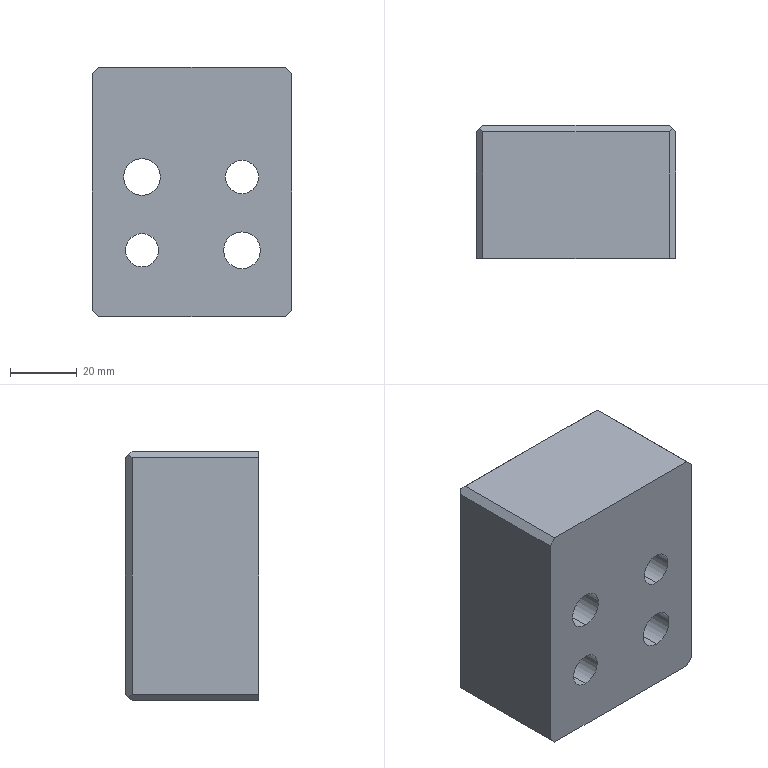Part | Creo | 1 solid | 28 faces | box 60 x 40 x 75 mm | volume 162492 mm3 | plane 16 | cylinder 12 | commonest cylinder face diameters 10 x4 11 x4 16.8 x4
STEP:
#1=CARTESIAN_POINT('',(-118.,350.,-254.5));
#2=VERTEX_POINT('',#1);
#3=CARTESIAN_POINT('',(-118.,350.,-243.5));
#4=VERTEX_POINT('',#3);
#5=CARTESIAN_POINT('',(-118.,350.,-249.));
#6=DIRECTION('',(0.,1.,0.));
#7=DIRECTION('',(0.,0.,-1.));
#8=AXIS2_PLACEMENT_3D('',#5,#6,#7);
#9=CIRCLE('',#8,5.5);
#10=EDGE_CURVE('',#2,#4,#9,.T.);
#11=ORIENTED_EDGE('',*,*,#10,.T.);
#12=CARTESIAN_POINT('',(-118.,379.,-243.5));
#13=VERTEX_POINT('',#12);
#14=CARTESIAN_POINT('',(-118.,350.,-243.5));
#15=DIRECTION('',(0.,1.,0.));
#16=VECTOR('',#15,29.);
#17=LINE('',#14,#16);
#18=EDGE_CURVE('',#4,#13,#17,.T.);
#19=ORIENTED_EDGE('',*,*,#18,.T.);
#20=CARTESIAN_POINT('',(-118.,379.,-254.5));
#21=VERTEX_POINT('',#20);
#22=CARTESIAN_POINT('',(-118.,379.,-249.));
#23=DIRECTION('',(0.,-1.,0.));
#24=DIRECTION('',(0.,0.,1.));
#25=AXIS2_PLACEMENT_3D('',#22,#23,#24);
#26=CIRCLE('',#25,5.5);
#27=EDGE_CURVE('',#13,#21,#26,.T.);
#28=ORIENTED_EDGE('',*,*,#27,.T.);
#29=CARTESIAN_POINT('',(-118.,350.,-254.5));
#30=DIRECTION('',(0.,1.,0.));
#31=VECTOR('',#30,29.);
#32=LINE('',#29,#31);
#33=EDGE_CURVE('',#2,#21,#32,.T.);
#34=ORIENTED_EDGE('',*,*,#33,.F.);
#35=EDGE_LOOP('',(#11,#19,#28,#34));
#36=FACE_OUTER_BOUND('',#35,.F.);
#37=CARTESIAN_POINT('',(-118.,390.,-249.));
#38=DIRECTION('',(0.,1.,0.));
#39=DIRECTION('',(0.,0.,-1.));
#40=AXIS2_PLACEMENT_3D('',#37,#38,#39);
#41=CYLINDRICAL_SURFACE('',#40,5.5);
#42=ADVANCED_FACE('',(#36),#41,.F.);
#43=CARTESIAN_POINT('',(-73.,350.,-289.));
#44=VERTEX_POINT('',#43);
#45=CARTESIAN_POINT('',(-73.,350.,-218.));
#46=VERTEX_POINT('',#45);
#47=CARTESIAN_POINT('',(-73.,350.,-289.));
#48=DIRECTION('',(0.,0.,1.));
#49=VECTOR('',#48,71.);
#50=LINE('',#47,#49);
#51=EDGE_CURVE('',#44,#46,#50,.T.);
#52=ORIENTED_EDGE('',*,*,#51,.F.);
#53=CARTESIAN_POINT('',(-75.,350.,-291.));
#54=VERTEX_POINT('',#53);
#55=CARTESIAN_POINT('',(-75.,350.,-291.));
#56=DIRECTION('',(0.7071,0.,0.7071));
#57=VECTOR('',#56,2.828);
#58=LINE('',#55,#57);
#59=EDGE_CURVE('',#54,#44,#58,.T.);
#60=ORIENTED_EDGE('',*,*,#59,.F.);
#61=CARTESIAN_POINT('',(-131.,350.,-291.));
#62=VERTEX_POINT('',#61);
#63=CARTESIAN_POINT('',(-131.,350.,-291.));
#64=DIRECTION('',(1.,0.,0.));
#65=VECTOR('',#64,56.);
#66=LINE('',#63,#65);
#67=EDGE_CURVE('',#62,#54,#66,.T.);
#68=ORIENTED_EDGE('',*,*,#67,.F.);
#69=CARTESIAN_POINT('',(-133.,350.,-289.));
#70=VERTEX_POINT('',#69);
#71=CARTESIAN_POINT('',(-133.,350.,-289.));
#72=DIRECTION('',(0.7071,0.,-0.7071));
#73=VECTOR('',#72,2.828);
#74=LINE('',#71,#73);
#75=EDGE_CURVE('',#70,#62,#74,.T.);
#76=ORIENTED_EDGE('',*,*,#75,.F.);
#77=CARTESIAN_POINT('',(-133.,350.,-218.));
#78=VERTEX_POINT('',#77);
#79=CARTESIAN_POINT('',(-133.,350.,-218.));
#80=DIRECTION('',(0.,0.,-1.));
#81=VECTOR('',#80,71.);
#82=LINE('',#79,#81);
#83=EDGE_CURVE('',#78,#70,#82,.T.);
#84=ORIENTED_EDGE('',*,*,#83,.F.);
#85=CARTESIAN_POINT('',(-131.,350.,-216.));
#86=VERTEX_POINT('',#85);
#87=CARTESIAN_POINT('',(-131.,350.,-216.));
#88=DIRECTION('',(-0.7071,0.,-0.7071));
#89=VECTOR('',#88,2.828);
#90=LINE('',#87,#89);
#91=EDGE_CURVE('',#86,#78,#90,.T.);
#92=ORIENTED_EDGE('',*,*,#91,.F.);
#93=CARTESIAN_POINT('',(-75.,350.,-216.));
#94=VERTEX_POINT('',#93);
#95=CARTESIAN_POINT('',(-75.,350.,-216.));
#96=DIRECTION('',(-1.,0.,0.));
#97=VECTOR('',#96,56.);
#98=LINE('',#95,#97);
#99=EDGE_CURVE('',#94,#86,#98,.T.);
#100=ORIENTED_EDGE('',*,*,#99,.F.);
#101=CARTESIAN_POINT('',(-73.,350.,-218.));
#102=DIRECTION('',(-0.7071,0.,0.7071));
#103=VECTOR('',#102,2.828);
#104=LINE('',#101,#103);
#105=EDGE_CURVE('',#46,#94,#104,.T.);
#106=ORIENTED_EDGE('',*,*,#105,.F.);
#107=EDGE_LOOP('',(#52,#60,#68,#76,#84,#92,#100,#106));
#108=FACE_OUTER_BOUND('',#107,.F.);
#109=ORIENTED_EDGE('',*,*,#10,.F.);
#110=CARTESIAN_POINT('',(-118.,350.,-249.));
#111=DIRECTION('',(0.,1.,0.));
#112=DIRECTION('',(0.,0.,1.));
#113=AXIS2_PLACEMENT_3D('',#110,#111,#112);
#114=CIRCLE('',#113,5.5);
#115=EDGE_CURVE('',#4,#2,#114,.T.);
#116=ORIENTED_EDGE('',*,*,#115,.F.);
#117=EDGE_LOOP('',(#109,#116));
#118=FACE_BOUND('',#117,.F.);
#119=CARTESIAN_POINT('',(-88.,350.,-276.5));
#120=VERTEX_POINT('',#119);
#121=CARTESIAN_POINT('',(-88.,350.,-265.5));
#122=VERTEX_POINT('',#121);
#123=CARTESIAN_POINT('',(-88.,350.,-271.));
#124=DIRECTION('',(0.,1.,0.));
#125=DIRECTION('',(0.,0.,-1.));
#126=AXIS2_PLACEMENT_3D('',#123,#124,#125);
#127=CIRCLE('',#126,5.5);
#128=EDGE_CURVE('',#120,#122,#127,.T.);
#129=ORIENTED_EDGE('',*,*,#128,.F.);
#130=CARTESIAN_POINT('',(-88.,350.,-271.));
#131=DIRECTION('',(0.,1.,0.));
#132=DIRECTION('',(0.,0.,1.));
#133=AXIS2_PLACEMENT_3D('',#130,#131,#132);
#134=CIRCLE('',#133,5.5);
#135=EDGE_CURVE('',#122,#120,#134,.T.);
#136=ORIENTED_EDGE('',*,*,#135,.F.);
#137=EDGE_LOOP('',(#129,#136));
#138=FACE_BOUND('',#137,.F.);
#139=CARTESIAN_POINT('',(-118.,350.,-276.));
#140=VERTEX_POINT('',#139);
#141=CARTESIAN_POINT('',(-118.,350.,-266.));
#142=VERTEX_POINT('',#141);
#143=CARTESIAN_POINT('',(-118.,350.,-271.));
#144=DIRECTION('',(0.,1.,0.));
#145=DIRECTION('',(0.,0.,-1.));
#146=AXIS2_PLACEMENT_3D('',#143,#144,#145);
#147=CIRCLE('',#146,5.);
#148=EDGE_CURVE('',#140,#142,#147,.T.);
#149=ORIENTED_EDGE('',*,*,#148,.F.);
#150=CARTESIAN_POINT('',(-118.,350.,-271.));
#151=DIRECTION('',(0.,1.,0.));
#152=DIRECTION('',(0.,0.,1.));
#153=AXIS2_PLACEMENT_3D('',#150,#151,#152);
#154=CIRCLE('',#153,5.);
#155=EDGE_CURVE('',#142,#140,#154,.T.);
#156=ORIENTED_EDGE('',*,*,#155,.F.);
#157=EDGE_LOOP('',(#149,#156));
#158=FACE_BOUND('',#157,.F.);
#159=CARTESIAN_POINT('',(-88.,350.,-254.));
#160=VERTEX_POINT('',#159);
#161=CARTESIAN_POINT('',(-88.,350.,-244.));
#162=VERTEX_POINT('',#161);
#163=CARTESIAN_POINT('',(-88.,350.,-249.));
#164=DIRECTION('',(0.,1.,0.));
#165=DIRECTION('',(0.,0.,-1.));
#166=AXIS2_PLACEMENT_3D('',#163,#164,#165);
#167=CIRCLE('',#166,5.);
#168=EDGE_CURVE('',#160,#162,#167,.T.);
#169=ORIENTED_EDGE('',*,*,#168,.F.);
#170=CARTESIAN_POINT('',(-88.,350.,-249.));
#171=DIRECTION('',(0.,1.,0.));
#172=DIRECTION('',(0.,0.,1.));
#173=AXIS2_PLACEMENT_3D('',#170,#171,#172);
#174=CIRCLE('',#173,5.);
#175=EDGE_CURVE('',#162,#160,#174,.T.);
#176=ORIENTED_EDGE('',*,*,#175,.F.);
#177=EDGE_LOOP('',(#169,#176));
#178=FACE_BOUND('',#177,.F.);
#179=CARTESIAN_POINT('',(321.5,350.,45.));
#180=DIRECTION('',(0.,1.,0.));
#181=DIRECTION('',(0.,0.,-1.));
#182=AXIS2_PLACEMENT_3D('',#179,#180,#181);
#183=PLANE('',#182);
#184=ADVANCED_FACE('',(#108,#118,#138,#158,#178),#183,.F.);
#185=CARTESIAN_POINT('',(-73.,388.,-289.));
#186=VERTEX_POINT('',#185);
#187=CARTESIAN_POINT('',(-73.,388.,-218.));
#188=VERTEX_POINT('',#187);
#189=CARTESIAN_POINT('',(-73.,388.,-289.));
#190=DIRECTION('',(0.,0.,1.));
#191=VECTOR('',#190,71.);
#192=LINE('',#189,#191);
#193=EDGE_CURVE('',#186,#188,#192,.T.);
#194=ORIENTED_EDGE('',*,*,#193,.F.);
#195=CARTESIAN_POINT('',(-73.,350.,-289.));
#196=DIRECTION('',(0.,1.,0.));
#197=VECTOR('',#196,38.);
#198=LINE('',#195,#197);
#199=EDGE_CURVE('',#44,#186,#198,.T.);
#200=ORIENTED_EDGE('',*,*,#199,.F.);
#201=ORIENTED_EDGE('',*,*,#51,.T.);
#202=CARTESIAN_POINT('',(-73.,350.,-218.));
#203=DIRECTION('',(0.,1.,0.));
#204=VECTOR('',#203,38.);
#205=LINE('',#202,#204);
#206=EDGE_CURVE('',#46,#188,#205,.T.);
#207=ORIENTED_EDGE('',*,*,#206,.T.);
#208=EDGE_LOOP('',(#194,#200,#201,#207));
#209=FACE_OUTER_BOUND('',#208,.F.);
#210=CARTESIAN_POINT('',(-73.,350.,-216.));
#211=DIRECTION('',(1.,0.,0.));
#212=DIRECTION('',(0.,0.,1.));
#213=AXIS2_PLACEMENT_3D('',#210,#211,#212);
#214=PLANE('',#213);
#215=ADVANCED_FACE('',(#209),#214,.T.);
#216=CARTESIAN_POINT('',(-74.,389.,-217.));
#217=VERTEX_POINT('',#216);
#218=CARTESIAN_POINT('',(-75.,390.,-218.));
#219=VERTEX_POINT('',#218);
#220=CARTESIAN_POINT('',(-74.,389.,-217.));
#221=DIRECTION('',(-0.5774,0.5774,-0.5774));
#222=VECTOR('',#221,1.732);
#223=LINE('',#220,#222);
#224=EDGE_CURVE('',#217,#219,#223,.T.);
#225=ORIENTED_EDGE('',*,*,#224,.T.);
#226=CARTESIAN_POINT('',(-75.,390.,-289.));
#227=VERTEX_POINT('',#226);
#228=CARTESIAN_POINT('',(-75.,390.,-289.));
#229=DIRECTION('',(0.,0.,1.));
#230=VECTOR('',#229,71.);
#231=LINE('',#228,#230);
#232=EDGE_CURVE('',#227,#219,#231,.T.);
#233=ORIENTED_EDGE('',*,*,#232,.F.);
#234=CARTESIAN_POINT('',(-74.,389.,-290.));
#235=VERTEX_POINT('',#234);
#236=CARTESIAN_POINT('',(-75.,390.,-289.));
#237=DIRECTION('',(0.5774,-0.5774,-0.5774));
#238=VECTOR('',#237,1.732);
#239=LINE('',#236,#238);
#240=EDGE_CURVE('',#227,#235,#239,.T.);
#241=ORIENTED_EDGE('',*,*,#240,.T.);
#242=CARTESIAN_POINT('',(-74.,389.,-290.));
#243=DIRECTION('',(0.5774,-0.5774,0.5774));
#244=VECTOR('',#243,1.732);
#245=LINE('',#242,#244);
#246=EDGE_CURVE('',#235,#186,#245,.T.);
#247=ORIENTED_EDGE('',*,*,#246,.T.);
#248=ORIENTED_EDGE('',*,*,#193,.T.);
#249=CARTESIAN_POINT('',(-74.,389.,-217.));
#250=DIRECTION('',(0.5774,-0.5774,-0.5774));
#251=VECTOR('',#250,1.732);
#252=LINE('',#249,#251);
#253=EDGE_CURVE('',#217,#188,#252,.T.);
#254=ORIENTED_EDGE('',*,*,#253,.F.);
#255=EDGE_LOOP('',(#225,#233,#241,#247,#248,#254));
#256=FACE_OUTER_BOUND('',#255,.F.);
#257=CARTESIAN_POINT('',(-74.,389.,-253.5));
#258=DIRECTION('',(0.7071,0.7071,0.));
#259=DIRECTION('',(-0.7071,0.7071,0.));
#260=AXIS2_PLACEMENT_3D('',#257,#258,#259);
#261=PLANE('',#260);
#262=ADVANCED_FACE('',(#256),#261,.T.);
#263=CARTESIAN_POINT('',(-75.,388.,-216.));
#264=VERTEX_POINT('',#263);
#265=CARTESIAN_POINT('',(-75.,388.,-216.));
#266=DIRECTION('',(0.5774,0.5774,-0.5774));
#267=VECTOR('',#266,1.732);
#268=LINE('',#265,#267);
#269=EDGE_CURVE('',#264,#217,#268,.T.);
#270=ORIENTED_EDGE('',*,*,#269,.F.);
#271=CARTESIAN_POINT('',(-131.,388.,-216.));
#272=VERTEX_POINT('',#271);
#273=CARTESIAN_POINT('',(-75.,388.,-216.));
#274=DIRECTION('',(-1.,0.,0.));
#275=VECTOR('',#274,56.);
#276=LINE('',#273,#275);
#277=EDGE_CURVE('',#264,#272,#276,.T.);
#278=ORIENTED_EDGE('',*,*,#277,.T.);
#279=CARTESIAN_POINT('',(-132.,389.,-217.));
#280=VERTEX_POINT('',#279);
#281=CARTESIAN_POINT('',(-132.,389.,-217.));
#282=DIRECTION('',(0.5774,-0.5774,0.5774));
#283=VECTOR('',#282,1.732);
#284=LINE('',#281,#283);
#285=EDGE_CURVE('',#280,#272,#284,.T.);
#286=ORIENTED_EDGE('',*,*,#285,.F.);
#287=CARTESIAN_POINT('',(-131.,390.,-218.));
#288=VERTEX_POINT('',#287);
#289=CARTESIAN_POINT('',(-132.,389.,-217.));
#290=DIRECTION('',(0.5774,0.5774,-0.5774));
#291=VECTOR('',#290,1.732);
#292=LINE('',#289,#291);
#293=EDGE_CURVE('',#280,#288,#292,.T.);
#294=ORIENTED_EDGE('',*,*,#293,.T.);
#295=CARTESIAN_POINT('',(-75.,390.,-218.));
#296=DIRECTION('',(-1.,0.,0.));
#297=VECTOR('',#296,56.);
#298=LINE('',#295,#297);
#299=EDGE_CURVE('',#219,#288,#298,.T.);
#300=ORIENTED_EDGE('',*,*,#299,.F.);
#301=ORIENTED_EDGE('',*,*,#224,.F.);
#302=EDGE_LOOP('',(#270,#278,#286,#294,#300,#301));
#303=FACE_OUTER_BOUND('',#302,.F.);
#304=CARTESIAN_POINT('',(-103.,389.,-217.));
#305=DIRECTION('',(0.,0.7071,0.7071));
#306=DIRECTION('',(0.,0.7071,-0.7071));
#307=AXIS2_PLACEMENT_3D('',#304,#305,#306);
#308=PLANE('',#307);
#309=ADVANCED_FACE('',(#303),#308,.T.);
#310=ORIENTED_EDGE('',*,*,#206,.F.);
#311=ORIENTED_EDGE('',*,*,#105,.T.);
#312=CARTESIAN_POINT('',(-75.,350.,-216.));
#313=DIRECTION('',(0.,1.,0.));
#314=VECTOR('',#313,38.);
#315=LINE('',#312,#314);
#316=EDGE_CURVE('',#94,#264,#315,.T.);
#317=ORIENTED_EDGE('',*,*,#316,.T.);
#318=ORIENTED_EDGE('',*,*,#269,.T.);
#319=ORIENTED_EDGE('',*,*,#253,.T.);
#320=EDGE_LOOP('',(#310,#311,#317,#318,#319));
#321=FACE_OUTER_BOUND('',#320,.F.);
#322=CARTESIAN_POINT('',(-74.,370.,-217.));
#323=DIRECTION('',(0.7071,0.,0.7071));
#324=DIRECTION('',(-0.7071,0.,0.7071));
#325=AXIS2_PLACEMENT_3D('',#322,#323,#324);
#326=PLANE('',#325);
#327=ADVANCED_FACE('',(#321),#326,.T.);
#328=ORIENTED_EDGE('',*,*,#99,.T.);
#329=CARTESIAN_POINT('',(-131.,350.,-216.));
#330=DIRECTION('',(0.,1.,0.));
#331=VECTOR('',#330,38.);
#332=LINE('',#329,#331);
#333=EDGE_CURVE('',#86,#272,#332,.T.);
#334=ORIENTED_EDGE('',*,*,#333,.T.);
#335=ORIENTED_EDGE('',*,*,#277,.F.);
#336=ORIENTED_EDGE('',*,*,#316,.F.);
#337=EDGE_LOOP('',(#328,#334,#335,#336));
#338=FACE_OUTER_BOUND('',#337,.F.);
#339=CARTESIAN_POINT('',(-133.,350.,-216.));
#340=DIRECTION('',(0.,0.,1.));
#341=DIRECTION('',(-1.,0.,0.));
#342=AXIS2_PLACEMENT_3D('',#339,#340,#341);
#343=PLANE('',#342);
#344=ADVANCED_FACE('',(#338),#343,.T.);
#345=ORIENTED_EDGE('',*,*,#333,.F.);
#346=ORIENTED_EDGE('',*,*,#91,.T.);
#347=CARTESIAN_POINT('',(-133.,388.,-218.));
#348=VERTEX_POINT('',#347);
#349=CARTESIAN_POINT('',(-133.,350.,-218.));
#350=DIRECTION('',(0.,1.,0.));
#351=VECTOR('',#350,38.);
#352=LINE('',#349,#351);
#353=EDGE_CURVE('',#78,#348,#352,.T.);
#354=ORIENTED_EDGE('',*,*,#353,.T.);
#355=CARTESIAN_POINT('',(-133.,388.,-218.));
#356=DIRECTION('',(0.5774,0.5774,0.5774));
#357=VECTOR('',#356,1.732);
#358=LINE('',#355,#357);
#359=EDGE_CURVE('',#348,#280,#358,.T.);
#360=ORIENTED_EDGE('',*,*,#359,.T.);
#361=ORIENTED_EDGE('',*,*,#285,.T.);
#362=EDGE_LOOP('',(#345,#346,#354,#360,#361));
#363=FACE_OUTER_BOUND('',#362,.F.);
#364=CARTESIAN_POINT('',(-132.,370.,-217.));
#365=DIRECTION('',(-0.7071,0.,0.7071));
#366=DIRECTION('',(-0.7071,0.,-0.7071));
#367=AXIS2_PLACEMENT_3D('',#364,#365,#366);
#368=PLANE('',#367);
#369=ADVANCED_FACE('',(#363),#368,.T.);
#370=ORIENTED_EDGE('',*,*,#83,.T.);
#371=CARTESIAN_POINT('',(-133.,388.,-289.));
#372=VERTEX_POINT('',#371);
#373=CARTESIAN_POINT('',(-133.,350.,-289.));
#374=DIRECTION('',(0.,1.,0.));
#375=VECTOR('',#374,38.);
#376=LINE('',#373,#375);
#377=EDGE_CURVE('',#70,#372,#376,.T.);
#378=ORIENTED_EDGE('',*,*,#377,.T.);
#379=CARTESIAN_POINT('',(-133.,388.,-218.));
#380=DIRECTION('',(0.,0.,-1.));
#381=VECTOR('',#380,71.);
#382=LINE('',#379,#381);
#383=EDGE_CURVE('',#348,#372,#382,.T.);
#384=ORIENTED_EDGE('',*,*,#383,.F.);
#385=ORIENTED_EDGE('',*,*,#353,.F.);
#386=EDGE_LOOP('',(#370,#378,#384,#385));
#387=FACE_OUTER_BOUND('',#386,.F.);
#388=CARTESIAN_POINT('',(-133.,350.,-291.));
#389=DIRECTION('',(-1.,0.,0.));
#390=DIRECTION('',(0.,0.,-1.));
#391=AXIS2_PLACEMENT_3D('',#388,#389,#390);
#392=PLANE('',#391);
#393=ADVANCED_FACE('',(#387),#392,.T.);
#394=ORIENTED_EDGE('',*,*,#377,.F.);
#395=ORIENTED_EDGE('',*,*,#75,.T.);
#396=CARTESIAN_POINT('',(-131.,388.,-291.));
#397=VERTEX_POINT('',#396);
#398=CARTESIAN_POINT('',(-131.,350.,-291.));
#399=DIRECTION('',(0.,1.,0.));
#400=VECTOR('',#399,38.);
#401=LINE('',#398,#400);
#402=EDGE_CURVE('',#62,#397,#401,.T.);
#403=ORIENTED_EDGE('',*,*,#402,.T.);
#404=CARTESIAN_POINT('',(-132.,389.,-290.));
#405=VERTEX_POINT('',#404);
#406=CARTESIAN_POINT('',(-131.,388.,-291.));
#407=DIRECTION('',(-0.5774,0.5774,0.5774));
#408=VECTOR('',#407,1.732);
#409=LINE('',#406,#408);
#410=EDGE_CURVE('',#397,#405,#409,.T.);
#411=ORIENTED_EDGE('',*,*,#410,.T.);
#412=CARTESIAN_POINT('',(-132.,389.,-290.));
#413=DIRECTION('',(-0.5774,-0.5774,0.5774));
#414=VECTOR('',#413,1.732);
#415=LINE('',#412,#414);
#416=EDGE_CURVE('',#405,#372,#415,.T.);
#417=ORIENTED_EDGE('',*,*,#416,.T.);
#418=EDGE_LOOP('',(#394,#395,#403,#411,#417));
#419=FACE_OUTER_BOUND('',#418,.F.);
#420=CARTESIAN_POINT('',(-132.,370.,-290.));
#421=DIRECTION('',(-0.7071,0.,-0.7071));
#422=DIRECTION('',(0.7071,0.,-0.7071));
#423=AXIS2_PLACEMENT_3D('',#420,#421,#422);
#424=PLANE('',#423);
#425=ADVANCED_FACE('',(#419),#424,.T.);
#426=ORIENTED_EDGE('',*,*,#67,.T.);
#427=CARTESIAN_POINT('',(-75.,388.,-291.));
#428=VERTEX_POINT('',#427);
#429=CARTESIAN_POINT('',(-75.,350.,-291.));
#430=DIRECTION('',(0.,1.,0.));
#431=VECTOR('',#430,38.);
#432=LINE('',#429,#431);
#433=EDGE_CURVE('',#54,#428,#432,.T.);
#434=ORIENTED_EDGE('',*,*,#433,.T.);
#435=CARTESIAN_POINT('',(-131.,388.,-291.));
#436=DIRECTION('',(1.,0.,0.));
#437=VECTOR('',#436,56.);
#438=LINE('',#435,#437);
#439=EDGE_CURVE('',#397,#428,#438,.T.);
#440=ORIENTED_EDGE('',*,*,#439,.F.);
#441=ORIENTED_EDGE('',*,*,#402,.F.);
#442=EDGE_LOOP('',(#426,#434,#440,#441));
#443=FACE_OUTER_BOUND('',#442,.F.);
#444=CARTESIAN_POINT('',(-73.,350.,-291.));
#445=DIRECTION('',(0.,0.,-1.));
#446=DIRECTION('',(1.,0.,0.));
#447=AXIS2_PLACEMENT_3D('',#444,#445,#446);
#448=PLANE('',#447);
#449=ADVANCED_FACE('',(#443),#448,.T.);
#450=ORIENTED_EDGE('',*,*,#433,.F.);
#451=ORIENTED_EDGE('',*,*,#59,.T.);
#452=ORIENTED_EDGE('',*,*,#199,.T.);
#453=ORIENTED_EDGE('',*,*,#246,.F.);
#454=CARTESIAN_POINT('',(-74.,389.,-290.));
#455=DIRECTION('',(-0.5774,-0.5774,-0.5774));
#456=VECTOR('',#455,1.732);
#457=LINE('',#454,#456);
#458=EDGE_CURVE('',#235,#428,#457,.T.);
#459=ORIENTED_EDGE('',*,*,#458,.T.);
#460=EDGE_LOOP('',(#450,#451,#452,#453,#459));
#461=FACE_OUTER_BOUND('',#460,.F.);
#462=CARTESIAN_POINT('',(-74.,370.,-290.));
#463=DIRECTION('',(0.7071,0.,-0.7071));
#464=DIRECTION('',(0.7071,0.,0.7071));
#465=AXIS2_PLACEMENT_3D('',#462,#463,#464);
#466=PLANE('',#465);
#467=ADVANCED_FACE('',(#461),#466,.T.);
#468=ORIENTED_EDGE('',*,*,#410,.F.);
#469=ORIENTED_EDGE('',*,*,#439,.T.);
#470=ORIENTED_EDGE('',*,*,#458,.F.);
#471=ORIENTED_EDGE('',*,*,#240,.F.);
#472=CARTESIAN_POINT('',(-131.,390.,-289.));
#473=VERTEX_POINT('',#472);
#474=CARTESIAN_POINT('',(-131.,390.,-289.));
#475=DIRECTION('',(1.,0.,0.));
#476=VECTOR('',#475,56.);
#477=LINE('',#474,#476);
#478=EDGE_CURVE('',#473,#227,#477,.T.);
#479=ORIENTED_EDGE('',*,*,#478,.F.);
#480=CARTESIAN_POINT('',(-132.,389.,-290.));
#481=DIRECTION('',(0.5774,0.5774,0.5774));
#482=VECTOR('',#481,1.732);
#483=LINE('',#480,#482);
#484=EDGE_CURVE('',#405,#473,#483,.T.);
#485=ORIENTED_EDGE('',*,*,#484,.F.);
#486=EDGE_LOOP('',(#468,#469,#470,#471,#479,#485));
#487=FACE_OUTER_BOUND('',#486,.F.);
#488=CARTESIAN_POINT('',(-103.,389.,-290.));
#489=DIRECTION('',(0.,0.7071,-0.7071));
#490=DIRECTION('',(0.,-0.7071,-0.7071));
#491=AXIS2_PLACEMENT_3D('',#488,#489,#490);
#492=PLANE('',#491);
#493=ADVANCED_FACE('',(#487),#492,.T.);
#494=ORIENTED_EDGE('',*,*,#299,.T.);
#495=CARTESIAN_POINT('',(-131.,390.,-218.));
#496=DIRECTION('',(0.,0.,-1.));
#497=VECTOR('',#496,71.);
#498=LINE('',#495,#497);
#499=EDGE_CURVE('',#288,#473,#498,.T.);
#500=ORIENTED_EDGE('',*,*,#499,.T.);
#501=ORIENTED_EDGE('',*,*,#478,.T.);
#502=ORIENTED_EDGE('',*,*,#232,.T.);
#503=EDGE_LOOP('',(#494,#500,#501,#502));
#504=FACE_OUTER_BOUND('',#503,.F.);
#505=CARTESIAN_POINT('',(-126.4,390.,-249.));
#506=VERTEX_POINT('',#505);
#507=CARTESIAN_POINT('',(-118.,390.,-257.4));
#508=VERTEX_POINT('',#507);
#509=CARTESIAN_POINT('',(-118.,390.,-249.));
#510=DIRECTION('',(0.,-1.,0.));
#511=DIRECTION('',(-1.,0.,0.));
#512=AXIS2_PLACEMENT_3D('',#509,#510,#511);
#513=CIRCLE('',#512,8.4);
#514=EDGE_CURVE('',#506,#508,#513,.T.);
#515=ORIENTED_EDGE('',*,*,#514,.F.);
#516=CARTESIAN_POINT('',(-118.,390.,-240.6));
#517=VERTEX_POINT('',#516);
#518=CARTESIAN_POINT('',(-118.,390.,-249.));
#519=DIRECTION('',(0.,-1.,0.));
#520=DIRECTION('',(0.,0.,1.));
#521=AXIS2_PLACEMENT_3D('',#518,#519,#520);
#522=CIRCLE('',#521,8.4);
#523=EDGE_CURVE('',#517,#506,#522,.T.);
#524=ORIENTED_EDGE('',*,*,#523,.F.);
#525=CARTESIAN_POINT('',(-118.,390.,-249.));
#526=DIRECTION('',(0.,-1.,0.));
#527=DIRECTION('',(0.,0.,-1.));
#528=AXIS2_PLACEMENT_3D('',#525,#526,#527);
#529=CIRCLE('',#528,8.4);
#530=EDGE_CURVE('',#508,#517,#529,.T.);
#531=ORIENTED_EDGE('',*,*,#530,.F.);
#532=EDGE_LOOP('',(#515,#524,#531));
#533=FACE_BOUND('',#532,.F.);
#534=CARTESIAN_POINT('',(-96.4,390.,-271.));
#535=VERTEX_POINT('',#534);
#536=CARTESIAN_POINT('',(-88.,390.,-279.4));
#537=VERTEX_POINT('',#536);
#538=CARTESIAN_POINT('',(-88.,390.,-271.));
#539=DIRECTION('',(0.,-1.,0.));
#540=DIRECTION('',(-1.,0.,0.));
#541=AXIS2_PLACEMENT_3D('',#538,#539,#540);
#542=CIRCLE('',#541,8.4);
#543=EDGE_CURVE('',#535,#537,#542,.T.);
#544=ORIENTED_EDGE('',*,*,#543,.F.);
#545=CARTESIAN_POINT('',(-88.,390.,-262.6));
#546=VERTEX_POINT('',#545);
#547=CARTESIAN_POINT('',(-88.,390.,-271.));
#548=DIRECTION('',(0.,-1.,0.));
#549=DIRECTION('',(0.,0.,1.));
#550=AXIS2_PLACEMENT_3D('',#547,#548,#549);
#551=CIRCLE('',#550,8.4);
#552=EDGE_CURVE('',#546,#535,#551,.T.);
#553=ORIENTED_EDGE('',*,*,#552,.F.);
#554=CARTESIAN_POINT('',(-88.,390.,-271.));
#555=DIRECTION('',(0.,-1.,0.));
#556=DIRECTION('',(0.,0.,-1.));
#557=AXIS2_PLACEMENT_3D('',#554,#555,#556);
#558=CIRCLE('',#557,8.4);
#559=EDGE_CURVE('',#537,#546,#558,.T.);
#560=ORIENTED_EDGE('',*,*,#559,.F.);
#561=EDGE_LOOP('',(#544,#553,#560));
#562=FACE_BOUND('',#561,.F.);
#563=CARTESIAN_POINT('',(-118.,390.,-276.));
#564=VERTEX_POINT('',#563);
#565=CARTESIAN_POINT('',(-118.,390.,-266.));
#566=VERTEX_POINT('',#565);
#567=CARTESIAN_POINT('',(-118.,390.,-271.));
#568=DIRECTION('',(0.,-1.,0.));
#569=DIRECTION('',(0.,0.,-1.));
#570=AXIS2_PLACEMENT_3D('',#567,#568,#569);
#571=CIRCLE('',#570,5.);
#572=EDGE_CURVE('',#564,#566,#571,.T.);
#573=ORIENTED_EDGE('',*,*,#572,.F.);
#574=CARTESIAN_POINT('',(-118.,390.,-271.));
#575=DIRECTION('',(0.,-1.,0.));
#576=DIRECTION('',(0.,0.,1.));
#577=AXIS2_PLACEMENT_3D('',#574,#575,#576);
#578=CIRCLE('',#577,5.);
#579=EDGE_CURVE('',#566,#564,#578,.T.);
#580=ORIENTED_EDGE('',*,*,#579,.F.);
#581=EDGE_LOOP('',(#573,#580));
#582=FACE_BOUND('',#581,.F.);
#583=CARTESIAN_POINT('',(-88.,390.,-254.));
#584=VERTEX_POINT('',#583);
#585=CARTESIAN_POINT('',(-88.,390.,-244.));
#586=VERTEX_POINT('',#585);
#587=CARTESIAN_POINT('',(-88.,390.,-249.));
#588=DIRECTION('',(0.,-1.,0.));
#589=DIRECTION('',(0.,0.,-1.));
#590=AXIS2_PLACEMENT_3D('',#587,#588,#589);
#591=CIRCLE('',#590,5.);
#592=EDGE_CURVE('',#584,#586,#591,.T.);
#593=ORIENTED_EDGE('',*,*,#592,.F.);
#594=CARTESIAN_POINT('',(-88.,390.,-249.));
#595=DIRECTION('',(0.,-1.,0.));
#596=DIRECTION('',(0.,0.,1.));
#597=AXIS2_PLACEMENT_3D('',#594,#595,#596);
#598=CIRCLE('',#597,5.);
#599=EDGE_CURVE('',#586,#584,#598,.T.);
#600=ORIENTED_EDGE('',*,*,#599,.F.);
#601=EDGE_LOOP('',(#593,#600));
#602=FACE_BOUND('',#601,.F.);
#603=CARTESIAN_POINT('',(321.5,390.,45.));
#604=DIRECTION('',(0.,1.,0.));
#605=DIRECTION('',(0.,0.,-1.));
#606=AXIS2_PLACEMENT_3D('',#603,#604,#605);
#607=PLANE('',#606);
#608=ADVANCED_FACE('',(#504,#533,#562,#582,#602),#607,.T.);
#609=ORIENTED_EDGE('',*,*,#552,.T.);
#610=ORIENTED_EDGE('',*,*,#543,.T.);
#611=CARTESIAN_POINT('',(-88.,379.,-279.4));
#612=VERTEX_POINT('',#611);
#613=CARTESIAN_POINT('',(-88.,379.,-279.4));
#614=DIRECTION('',(0.,1.,0.));
#615=VECTOR('',#614,11.);
#616=LINE('',#613,#615);
#617=EDGE_CURVE('',#612,#537,#616,.T.);
#618=ORIENTED_EDGE('',*,*,#617,.F.);
#619=CARTESIAN_POINT('',(-96.4,379.,-271.));
#620=VERTEX_POINT('',#619);
#621=CARTESIAN_POINT('',(-88.,379.,-271.));
#622=DIRECTION('',(0.,1.,0.));
#623=DIRECTION('',(0.,0.,-1.));
#624=AXIS2_PLACEMENT_3D('',#621,#622,#623);
#625=CIRCLE('',#624,8.4);
#626=EDGE_CURVE('',#612,#620,#625,.T.);
#627=ORIENTED_EDGE('',*,*,#626,.T.);
#628=CARTESIAN_POINT('',(-88.,379.,-262.6));
#629=VERTEX_POINT('',#628);
#630=CARTESIAN_POINT('',(-88.,379.,-271.));
#631=DIRECTION('',(0.,1.,0.));
#632=DIRECTION('',(-1.,0.,0.));
#633=AXIS2_PLACEMENT_3D('',#630,#631,#632);
#634=CIRCLE('',#633,8.4);
#635=EDGE_CURVE('',#620,#629,#634,.T.);
#636=ORIENTED_EDGE('',*,*,#635,.T.);
#637=CARTESIAN_POINT('',(-88.,379.,-262.6));
#638=DIRECTION('',(0.,1.,0.));
#639=VECTOR('',#638,11.);
#640=LINE('',#637,#639);
#641=EDGE_CURVE('',#629,#546,#640,.T.);
#642=ORIENTED_EDGE('',*,*,#641,.T.);
#643=EDGE_LOOP('',(#609,#610,#618,#627,#636,#642));
#644=FACE_OUTER_BOUND('',#643,.F.);
#645=CARTESIAN_POINT('',(-88.,379.,-271.));
#646=DIRECTION('',(0.,1.,0.));
#647=DIRECTION('',(0.,0.,-1.));
#648=AXIS2_PLACEMENT_3D('',#645,#646,#647);
#649=CYLINDRICAL_SURFACE('',#648,8.4);
#650=ADVANCED_FACE('',(#644),#649,.F.);
#651=ORIENTED_EDGE('',*,*,#559,.T.);
#652=ORIENTED_EDGE('',*,*,#641,.F.);
#653=CARTESIAN_POINT('',(-79.6,379.,-271.));
#654=VERTEX_POINT('',#653);
#655=CARTESIAN_POINT('',(-88.,379.,-271.));
#656=DIRECTION('',(0.,1.,0.));
#657=DIRECTION('',(0.,0.,1.));
#658=AXIS2_PLACEMENT_3D('',#655,#656,#657);
#659=CIRCLE('',#658,8.4);
#660=EDGE_CURVE('',#629,#654,#659,.T.);
#661=ORIENTED_EDGE('',*,*,#660,.T.);
#662=CARTESIAN_POINT('',(-88.,379.,-271.));
#663=DIRECTION('',(0.,1.,0.));
#664=DIRECTION('',(1.,0.,0.));
#665=AXIS2_PLACEMENT_3D('',#662,#663,#664);
#666=CIRCLE('',#665,8.4);
#667=EDGE_CURVE('',#654,#612,#666,.T.);
#668=ORIENTED_EDGE('',*,*,#667,.T.);
#669=ORIENTED_EDGE('',*,*,#617,.T.);
#670=EDGE_LOOP('',(#651,#652,#661,#668,#669));
#671=FACE_OUTER_BOUND('',#670,.F.);
#672=CARTESIAN_POINT('',(-88.,379.,-271.));
#673=DIRECTION('',(0.,1.,0.));
#674=DIRECTION('',(0.,0.,-1.));
#675=AXIS2_PLACEMENT_3D('',#672,#673,#674);
#676=CYLINDRICAL_SURFACE('',#675,8.4);
#677=ADVANCED_FACE('',(#671),#676,.F.);
#678=ORIENTED_EDGE('',*,*,#635,.F.);
#679=ORIENTED_EDGE('',*,*,#626,.F.);
#680=ORIENTED_EDGE('',*,*,#667,.F.);
#681=ORIENTED_EDGE('',*,*,#660,.F.);
#682=EDGE_LOOP('',(#678,#679,#680,#681));
#683=FACE_OUTER_BOUND('',#682,.F.);
#684=CARTESIAN_POINT('',(-88.,379.,-276.5));
#685=VERTEX_POINT('',#684);
#686=CARTESIAN_POINT('',(-88.,379.,-265.5));
#687=VERTEX_POINT('',#686);
#688=CARTESIAN_POINT('',(-88.,379.,-271.));
#689=DIRECTION('',(0.,-1.,0.));
#690=DIRECTION('',(0.,0.,-1.));
#691=AXIS2_PLACEMENT_3D('',#688,#689,#690);
#692=CIRCLE('',#691,5.5);
#693=EDGE_CURVE('',#685,#687,#692,.T.);
#694=ORIENTED_EDGE('',*,*,#693,.F.);
#695=CARTESIAN_POINT('',(-88.,379.,-271.));
#696=DIRECTION('',(0.,-1.,0.));
#697=DIRECTION('',(0.,0.,1.));
#698=AXIS2_PLACEMENT_3D('',#695,#696,#697);
#699=CIRCLE('',#698,5.5);
#700=EDGE_CURVE('',#687,#685,#699,.T.);
#701=ORIENTED_EDGE('',*,*,#700,.F.);
#702=EDGE_LOOP('',(#694,#701));
#703=FACE_BOUND('',#702,.F.);
#704=CARTESIAN_POINT('',(21.5,379.,49.5));
#705=DIRECTION('',(0.,1.,0.));
#706=DIRECTION('',(0.,0.,-1.));
#707=AXIS2_PLACEMENT_3D('',#704,#705,#706);
#708=PLANE('',#707);
#709=ADVANCED_FACE('',(#683,#703),#708,.T.);
#710=ORIENTED_EDGE('',*,*,#135,.T.);
#711=CARTESIAN_POINT('',(-88.,350.,-276.5));
#712=DIRECTION('',(0.,1.,0.));
#713=VECTOR('',#712,29.);
#714=LINE('',#711,#713);
#715=EDGE_CURVE('',#120,#685,#714,.T.);
#716=ORIENTED_EDGE('',*,*,#715,.T.);
#717=ORIENTED_EDGE('',*,*,#693,.T.);
#718=CARTESIAN_POINT('',(-88.,350.,-265.5));
#719=DIRECTION('',(0.,1.,0.));
#720=VECTOR('',#719,29.);
#721=LINE('',#718,#720);
#722=EDGE_CURVE('',#122,#687,#721,.T.);
#723=ORIENTED_EDGE('',*,*,#722,.F.);
#724=EDGE_LOOP('',(#710,#716,#717,#723));
#725=FACE_OUTER_BOUND('',#724,.F.);
#726=CARTESIAN_POINT('',(-88.,390.,-271.));
#727=DIRECTION('',(0.,1.,0.));
#728=DIRECTION('',(0.,0.,-1.));
#729=AXIS2_PLACEMENT_3D('',#726,#727,#728);
#730=CYLINDRICAL_SURFACE('',#729,5.5);
#731=ADVANCED_FACE('',(#725),#730,.F.);
#732=ORIENTED_EDGE('',*,*,#128,.T.);
#733=ORIENTED_EDGE('',*,*,#722,.T.);
#734=ORIENTED_EDGE('',*,*,#700,.T.);
#735=ORIENTED_EDGE('',*,*,#715,.F.);
#736=EDGE_LOOP('',(#732,#733,#734,#735));
#737=FACE_OUTER_BOUND('',#736,.F.);
#738=CARTESIAN_POINT('',(-88.,390.,-271.));
#739=DIRECTION('',(0.,1.,0.));
#740=DIRECTION('',(0.,0.,-1.));
#741=AXIS2_PLACEMENT_3D('',#738,#739,#740);
#742=CYLINDRICAL_SURFACE('',#741,5.5);
#743=ADVANCED_FACE('',(#737),#742,.F.);
#744=ORIENTED_EDGE('',*,*,#523,.T.);
#745=ORIENTED_EDGE('',*,*,#514,.T.);
#746=CARTESIAN_POINT('',(-118.,379.,-257.4));
#747=VERTEX_POINT('',#746);
#748=CARTESIAN_POINT('',(-118.,379.,-257.4));
#749=DIRECTION('',(0.,1.,0.));
#750=VECTOR('',#749,11.);
#751=LINE('',#748,#750);
#752=EDGE_CURVE('',#747,#508,#751,.T.);
#753=ORIENTED_EDGE('',*,*,#752,.F.);
#754=CARTESIAN_POINT('',(-126.4,379.,-249.));
#755=VERTEX_POINT('',#754);
#756=CARTESIAN_POINT('',(-118.,379.,-249.));
#757=DIRECTION('',(0.,1.,0.));
#758=DIRECTION('',(0.,0.,-1.));
#759=AXIS2_PLACEMENT_3D('',#756,#757,#758);
#760=CIRCLE('',#759,8.4);
#761=EDGE_CURVE('',#747,#755,#760,.T.);
#762=ORIENTED_EDGE('',*,*,#761,.T.);
#763=CARTESIAN_POINT('',(-118.,379.,-240.6));
#764=VERTEX_POINT('',#763);
#765=CARTESIAN_POINT('',(-118.,379.,-249.));
#766=DIRECTION('',(0.,1.,0.));
#767=DIRECTION('',(-1.,0.,0.));
#768=AXIS2_PLACEMENT_3D('',#765,#766,#767);
#769=CIRCLE('',#768,8.4);
#770=EDGE_CURVE('',#755,#764,#769,.T.);
#771=ORIENTED_EDGE('',*,*,#770,.T.);
#772=CARTESIAN_POINT('',(-118.,379.,-240.6));
#773=DIRECTION('',(0.,1.,0.));
#774=VECTOR('',#773,11.);
#775=LINE('',#772,#774);
#776=EDGE_CURVE('',#764,#517,#775,.T.);
#777=ORIENTED_EDGE('',*,*,#776,.T.);
#778=EDGE_LOOP('',(#744,#745,#753,#762,#771,#777));
#779=FACE_OUTER_BOUND('',#778,.F.);
#780=CARTESIAN_POINT('',(-118.,379.,-249.));
#781=DIRECTION('',(0.,1.,0.));
#782=DIRECTION('',(0.,0.,-1.));
#783=AXIS2_PLACEMENT_3D('',#780,#781,#782);
#784=CYLINDRICAL_SURFACE('',#783,8.4);
#785=ADVANCED_FACE('',(#779),#784,.F.);
#786=ORIENTED_EDGE('',*,*,#530,.T.);
#787=ORIENTED_EDGE('',*,*,#776,.F.);
#788=CARTESIAN_POINT('',(-109.6,379.,-249.));
#789=VERTEX_POINT('',#788);
#790=CARTESIAN_POINT('',(-118.,379.,-249.));
#791=DIRECTION('',(0.,1.,0.));
#792=DIRECTION('',(0.,0.,1.));
#793=AXIS2_PLACEMENT_3D('',#790,#791,#792);
#794=CIRCLE('',#793,8.4);
#795=EDGE_CURVE('',#764,#789,#794,.T.);
#796=ORIENTED_EDGE('',*,*,#795,.T.);
#797=CARTESIAN_POINT('',(-118.,379.,-249.));
#798=DIRECTION('',(0.,1.,0.));
#799=DIRECTION('',(1.,0.,0.));
#800=AXIS2_PLACEMENT_3D('',#797,#798,#799);
#801=CIRCLE('',#800,8.4);
#802=EDGE_CURVE('',#789,#747,#801,.T.);
#803=ORIENTED_EDGE('',*,*,#802,.T.);
#804=ORIENTED_EDGE('',*,*,#752,.T.);
#805=EDGE_LOOP('',(#786,#787,#796,#803,#804));
#806=FACE_OUTER_BOUND('',#805,.F.);
#807=CARTESIAN_POINT('',(-118.,379.,-249.));
#808=DIRECTION('',(0.,1.,0.));
#809=DIRECTION('',(0.,0.,-1.));
#810=AXIS2_PLACEMENT_3D('',#807,#808,#809);
#811=CYLINDRICAL_SURFACE('',#810,8.4);
#812=ADVANCED_FACE('',(#806),#811,.F.);
#813=ORIENTED_EDGE('',*,*,#770,.F.);
#814=ORIENTED_EDGE('',*,*,#761,.F.);
#815=ORIENTED_EDGE('',*,*,#802,.F.);
#816=ORIENTED_EDGE('',*,*,#795,.F.);
#817=EDGE_LOOP('',(#813,#814,#815,#816));
#818=FACE_OUTER_BOUND('',#817,.F.);
#819=CARTESIAN_POINT('',(-118.,379.,-249.));
#820=DIRECTION('',(0.,-1.,0.));
#821=DIRECTION('',(0.,0.,-1.));
#822=AXIS2_PLACEMENT_3D('',#819,#820,#821);
#823=CIRCLE('',#822,5.5);
#824=EDGE_CURVE('',#21,#13,#823,.T.);
#825=ORIENTED_EDGE('',*,*,#824,.F.);
#826=ORIENTED_EDGE('',*,*,#27,.F.);
#827=EDGE_LOOP('',(#825,#826));
#828=FACE_BOUND('',#827,.F.);
#829=CARTESIAN_POINT('',(21.5,379.,26.5));
#830=DIRECTION('',(0.,1.,0.));
#831=DIRECTION('',(0.,0.,-1.));
#832=AXIS2_PLACEMENT_3D('',#829,#830,#831);
#833=PLANE('',#832);
#834=ADVANCED_FACE('',(#818,#828),#833,.T.);
#835=ORIENTED_EDGE('',*,*,#115,.T.);
#836=ORIENTED_EDGE('',*,*,#33,.T.);
#837=ORIENTED_EDGE('',*,*,#824,.T.);
#838=ORIENTED_EDGE('',*,*,#18,.F.);
#839=EDGE_LOOP('',(#835,#836,#837,#838));
#840=FACE_OUTER_BOUND('',#839,.F.);
#841=CARTESIAN_POINT('',(-118.,390.,-249.));
#842=DIRECTION('',(0.,1.,0.));
#843=DIRECTION('',(0.,0.,-1.));
#844=AXIS2_PLACEMENT_3D('',#841,#842,#843);
#845=CYLINDRICAL_SURFACE('',#844,5.5);
#846=ADVANCED_FACE('',(#840),#845,.F.);
#847=ORIENTED_EDGE('',*,*,#359,.F.);
#848=ORIENTED_EDGE('',*,*,#383,.T.);
#849=ORIENTED_EDGE('',*,*,#416,.F.);
#850=ORIENTED_EDGE('',*,*,#484,.T.);
#851=ORIENTED_EDGE('',*,*,#499,.F.);
#852=ORIENTED_EDGE('',*,*,#293,.F.);
#853=EDGE_LOOP('',(#847,#848,#849,#850,#851,#852));
#854=FACE_OUTER_BOUND('',#853,.F.);
#855=CARTESIAN_POINT('',(-132.,389.,-253.5));
#856=DIRECTION('',(-0.7071,0.7071,0.));
#857=DIRECTION('',(-0.7071,-0.7071,0.));
#858=AXIS2_PLACEMENT_3D('',#855,#856,#857);
#859=PLANE('',#858);
#860=ADVANCED_FACE('',(#854),#859,.T.);
#861=ORIENTED_EDGE('',*,*,#155,.T.);
#862=CARTESIAN_POINT('',(-118.,350.,-276.));
#863=DIRECTION('',(0.,1.,0.));
#864=VECTOR('',#863,40.);
#865=LINE('',#862,#864);
#866=EDGE_CURVE('',#140,#564,#865,.T.);
#867=ORIENTED_EDGE('',*,*,#866,.T.);
#868=ORIENTED_EDGE('',*,*,#572,.T.);
#869=CARTESIAN_POINT('',(-118.,350.,-266.));
#870=DIRECTION('',(0.,1.,0.));
#871=VECTOR('',#870,40.);
#872=LINE('',#869,#871);
#873=EDGE_CURVE('',#142,#566,#872,.T.);
#874=ORIENTED_EDGE('',*,*,#873,.F.);
#875=EDGE_LOOP('',(#861,#867,#868,#874));
#876=FACE_OUTER_BOUND('',#875,.F.);
#877=CARTESIAN_POINT('',(-118.,662.866,-271.));
#878=DIRECTION('',(0.,1.,0.));
#879=DIRECTION('',(0.,0.,-1.));
#880=AXIS2_PLACEMENT_3D('',#877,#878,#879);
#881=CYLINDRICAL_SURFACE('',#880,5.);
#882=ADVANCED_FACE('',(#876),#881,.F.);
#883=ORIENTED_EDGE('',*,*,#148,.T.);
#884=ORIENTED_EDGE('',*,*,#873,.T.);
#885=ORIENTED_EDGE('',*,*,#579,.T.);
#886=ORIENTED_EDGE('',*,*,#866,.F.);
#887=EDGE_LOOP('',(#883,#884,#885,#886));
#888=FACE_OUTER_BOUND('',#887,.F.);
#889=CARTESIAN_POINT('',(-118.,662.866,-271.));
#890=DIRECTION('',(0.,1.,0.));
#891=DIRECTION('',(0.,0.,-1.));
#892=AXIS2_PLACEMENT_3D('',#889,#890,#891);
#893=CYLINDRICAL_SURFACE('',#892,5.);
#894=ADVANCED_FACE('',(#888),#893,.F.);
#895=ORIENTED_EDGE('',*,*,#175,.T.);
#896=CARTESIAN_POINT('',(-88.,350.,-254.));
#897=DIRECTION('',(0.,1.,0.));
#898=VECTOR('',#897,40.);
#899=LINE('',#896,#898);
#900=EDGE_CURVE('',#160,#584,#899,.T.);
#901=ORIENTED_EDGE('',*,*,#900,.T.);
#902=ORIENTED_EDGE('',*,*,#592,.T.);
#903=CARTESIAN_POINT('',(-88.,350.,-244.));
#904=DIRECTION('',(0.,1.,0.));
#905=VECTOR('',#904,40.);
#906=LINE('',#903,#905);
#907=EDGE_CURVE('',#162,#586,#906,.T.);
#908=ORIENTED_EDGE('',*,*,#907,.F.);
#909=EDGE_LOOP('',(#895,#901,#902,#908));
#910=FACE_OUTER_BOUND('',#909,.F.);
#911=CARTESIAN_POINT('',(-88.,662.866,-249.));
#912=DIRECTION('',(0.,1.,0.));
#913=DIRECTION('',(0.,0.,-1.));
#914=AXIS2_PLACEMENT_3D('',#911,#912,#913);
#915=CYLINDRICAL_SURFACE('',#914,5.);
#916=ADVANCED_FACE('',(#910),#915,.F.);
#917=ORIENTED_EDGE('',*,*,#168,.T.);
#918=ORIENTED_EDGE('',*,*,#907,.T.);
#919=ORIENTED_EDGE('',*,*,#599,.T.);
#920=ORIENTED_EDGE('',*,*,#900,.F.);
#921=EDGE_LOOP('',(#917,#918,#919,#920));
#922=FACE_OUTER_BOUND('',#921,.F.);
#923=CARTESIAN_POINT('',(-88.,662.866,-249.));
#924=DIRECTION('',(0.,1.,0.));
#925=DIRECTION('',(0.,0.,-1.));
#926=AXIS2_PLACEMENT_3D('',#923,#924,#925);
#927=CYLINDRICAL_SURFACE('',#926,5.);
#928=ADVANCED_FACE('',(#922),#927,.F.);
#929=CLOSED_SHELL('',(#42,#184,#215,#262,#309,#327,#344,#369,#393,#425,#449,#467,#493,#608,#650,#677,#709,#731,#743,#785,#812,#834,#846,#860,#882,#894,#916,#928));
#930=MANIFOLD_SOLID_BREP('',#929);
#931=(LENGTH_UNIT()NAMED_UNIT(*)SI_UNIT(.MILLI.,.METRE.));
#932=UNCERTAINTY_MEASURE_WITH_UNIT(LENGTH_MEASURE(0.0104),#931,'','');
#933=(NAMED_UNIT(*)PLANE_ANGLE_UNIT()SI_UNIT($,.RADIAN.));
#934=PLANE_ANGLE_MEASURE_WITH_UNIT(PLANE_ANGLE_MEASURE(0.01745),#933);
#935=(CONVERSION_BASED_UNIT('DEGREE',#934)NAMED_UNIT(*)PLANE_ANGLE_UNIT());
#936=(NAMED_UNIT(*)SI_UNIT($,.STERADIAN.)SOLID_ANGLE_UNIT());
#937=(GEOMETRIC_REPRESENTATION_CONTEXT(3)GLOBAL_UNCERTAINTY_ASSIGNED_CONTEXT((#932))GLOBAL_UNIT_ASSIGNED_CONTEXT((#931,#935,#936))REPRESENTATION_CONTEXT('',''));
#938=ADVANCED_BREP_SHAPE_REPRESENTATION('',(#930),#937);